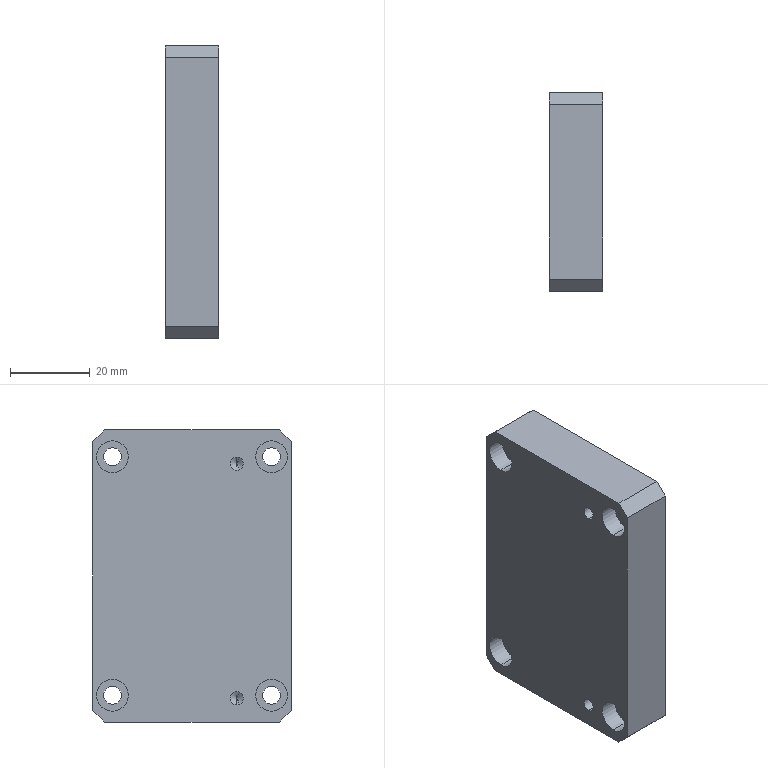Part | SolidWorks | features HoleWzd 3, Chamfer 1, Extrusion 1 | 1 solid | 46 faces | box 13.5 x 50 x 73.5 mm | volume 47539 mm3 | cylinder 24 | plane 14 | cone 8 | commonest cylinder face diameters 4.5 x8 8 x8 3.3 x4 4 x4
STEP:
#1=CARTESIAN_POINT('',(10.1,-11.25,26.6));
#2=VERTEX_POINT('',#1);
#3=CARTESIAN_POINT('',(10.1,-11.25,29.9));
#4=VERTEX_POINT('',#3);
#5=CARTESIAN_POINT('',(10.1,-11.25,28.25));
#6=DIRECTION('',(-1.,0.,0.));
#7=DIRECTION('',(0.,0.,1.));
#8=AXIS2_PLACEMENT_3D('',#5,#6,#7);
#9=CIRCLE('',#8,1.65);
#10=EDGE_CURVE('',#2,#4,#9,.T.);
#11=ORIENTED_EDGE('',*,*,#10,.F.);
#12=CARTESIAN_POINT('',(0.,-11.25,26.6));
#13=VERTEX_POINT('',#12);
#14=CARTESIAN_POINT('',(0.,-11.25,26.6));
#15=DIRECTION('',(-1.,0.,0.));
#16=VECTOR('',#15,1000.);
#17=LINE('',#14,#16);
#18=EDGE_CURVE('',#2,#13,#17,.T.);
#19=ORIENTED_EDGE('',*,*,#18,.T.);
#20=CARTESIAN_POINT('',(0.,-11.25,29.9));
#21=VERTEX_POINT('',#20);
#22=CARTESIAN_POINT('',(0.,-11.25,28.25));
#23=DIRECTION('',(-1.,0.,0.));
#24=DIRECTION('',(0.,0.,1.));
#25=AXIS2_PLACEMENT_3D('',#22,#23,#24);
#26=CIRCLE('',#25,1.65);
#27=EDGE_CURVE('',#13,#21,#26,.T.);
#28=ORIENTED_EDGE('',*,*,#27,.T.);
#29=CARTESIAN_POINT('',(0.,-11.25,29.9));
#30=DIRECTION('',(-1.,0.,0.));
#31=VECTOR('',#30,1000.);
#32=LINE('',#29,#31);
#33=EDGE_CURVE('',#4,#21,#32,.T.);
#34=ORIENTED_EDGE('',*,*,#33,.F.);
#35=EDGE_LOOP('',(#11,#19,#28,#34));
#36=FACE_OUTER_BOUND('',#35,.T.);
#37=CARTESIAN_POINT('',(0.,-11.25,28.25));
#38=DIRECTION('',(-1.,0.,0.));
#39=DIRECTION('',(0.,0.,1.));
#40=AXIS2_PLACEMENT_3D('',#37,#38,#39);
#41=CYLINDRICAL_SURFACE('',#40,1.65);
#42=ADVANCED_FACE('',(#36),#41,.F.);
#43=CARTESIAN_POINT('',(11.091,-11.25,28.25));
#44=VERTEX_POINT('',#43);
#45=CARTESIAN_POINT('',(10.1,-11.25,29.9));
#46=DIRECTION('',(-0.515,0.,0.8572));
#47=VECTOR('',#46,1000.);
#48=LINE('',#45,#47);
#49=EDGE_CURVE('',#44,#4,#48,.T.);
#50=ORIENTED_EDGE('',*,*,#49,.F.);
#51=CARTESIAN_POINT('',(10.1,-11.25,26.6));
#52=DIRECTION('',(-0.515,0.,-0.8572));
#53=VECTOR('',#52,1000.);
#54=LINE('',#51,#53);
#55=EDGE_CURVE('',#44,#2,#54,.T.);
#56=ORIENTED_EDGE('',*,*,#55,.T.);
#57=ORIENTED_EDGE('',*,*,#10,.T.);
#58=EDGE_LOOP('',(#50,#56,#57));
#59=FACE_OUTER_BOUND('',#58,.T.);
#60=CARTESIAN_POINT('',(10.1,-11.25,28.25));
#61=DIRECTION('',(-1.,0.,0.));
#62=DIRECTION('',(0.,0.,1.));
#63=AXIS2_PLACEMENT_3D('',#60,#61,#62);
#64=CONICAL_SURFACE('',#63,1.65,1.03);
#65=ADVANCED_FACE('',(#59),#64,.F.);
#66=CARTESIAN_POINT('',(10.1,-11.25,-32.4));
#67=VERTEX_POINT('',#66);
#68=CARTESIAN_POINT('',(10.1,-11.25,-29.1));
#69=VERTEX_POINT('',#68);
#70=CARTESIAN_POINT('',(10.1,-11.25,-30.75));
#71=DIRECTION('',(-1.,0.,0.));
#72=DIRECTION('',(0.,0.,1.));
#73=AXIS2_PLACEMENT_3D('',#70,#71,#72);
#74=CIRCLE('',#73,1.65);
#75=EDGE_CURVE('',#67,#69,#74,.T.);
#76=ORIENTED_EDGE('',*,*,#75,.F.);
#77=CARTESIAN_POINT('',(0.,-11.25,-32.4));
#78=VERTEX_POINT('',#77);
#79=CARTESIAN_POINT('',(0.,-11.25,-32.4));
#80=DIRECTION('',(-1.,0.,0.));
#81=VECTOR('',#80,1000.);
#82=LINE('',#79,#81);
#83=EDGE_CURVE('',#67,#78,#82,.T.);
#84=ORIENTED_EDGE('',*,*,#83,.T.);
#85=CARTESIAN_POINT('',(0.,-11.25,-29.1));
#86=VERTEX_POINT('',#85);
#87=CARTESIAN_POINT('',(0.,-11.25,-30.75));
#88=DIRECTION('',(-1.,0.,0.));
#89=DIRECTION('',(0.,0.,1.));
#90=AXIS2_PLACEMENT_3D('',#87,#88,#89);
#91=CIRCLE('',#90,1.65);
#92=EDGE_CURVE('',#78,#86,#91,.T.);
#93=ORIENTED_EDGE('',*,*,#92,.T.);
#94=CARTESIAN_POINT('',(0.,-11.25,-29.1));
#95=DIRECTION('',(-1.,0.,0.));
#96=VECTOR('',#95,1000.);
#97=LINE('',#94,#96);
#98=EDGE_CURVE('',#69,#86,#97,.T.);
#99=ORIENTED_EDGE('',*,*,#98,.F.);
#100=EDGE_LOOP('',(#76,#84,#93,#99));
#101=FACE_OUTER_BOUND('',#100,.T.);
#102=CARTESIAN_POINT('',(0.,-11.25,-30.75));
#103=DIRECTION('',(-1.,0.,0.));
#104=DIRECTION('',(0.,0.,1.));
#105=AXIS2_PLACEMENT_3D('',#102,#103,#104);
#106=CYLINDRICAL_SURFACE('',#105,1.65);
#107=ADVANCED_FACE('',(#101),#106,.F.);
#108=CARTESIAN_POINT('',(11.091,-11.25,-30.75));
#109=VERTEX_POINT('',#108);
#110=CARTESIAN_POINT('',(10.1,-11.25,-29.1));
#111=DIRECTION('',(-0.515,0.,0.8572));
#112=VECTOR('',#111,1000.);
#113=LINE('',#110,#112);
#114=EDGE_CURVE('',#109,#69,#113,.T.);
#115=ORIENTED_EDGE('',*,*,#114,.F.);
#116=CARTESIAN_POINT('',(10.1,-11.25,-32.4));
#117=DIRECTION('',(-0.515,0.,-0.8572));
#118=VECTOR('',#117,1000.);
#119=LINE('',#116,#118);
#120=EDGE_CURVE('',#109,#67,#119,.T.);
#121=ORIENTED_EDGE('',*,*,#120,.T.);
#122=ORIENTED_EDGE('',*,*,#75,.T.);
#123=EDGE_LOOP('',(#115,#121,#122));
#124=FACE_OUTER_BOUND('',#123,.T.);
#125=CARTESIAN_POINT('',(10.1,-11.25,-30.75));
#126=DIRECTION('',(-1.,0.,0.));
#127=DIRECTION('',(0.,0.,1.));
#128=AXIS2_PLACEMENT_3D('',#125,#126,#127);
#129=CONICAL_SURFACE('',#128,1.65,1.03);
#130=ADVANCED_FACE('',(#124),#129,.F.);
#131=CARTESIAN_POINT('',(7.5,0.,32.));
#132=VERTEX_POINT('',#131);
#133=CARTESIAN_POINT('',(7.5,0.,28.));
#134=VERTEX_POINT('',#133);
#135=CARTESIAN_POINT('',(7.5,0.,30.));
#136=DIRECTION('',(1.,0.,0.));
#137=DIRECTION('',(0.,0.,-1.));
#138=AXIS2_PLACEMENT_3D('',#135,#136,#137);
#139=CIRCLE('',#138,2.);
#140=EDGE_CURVE('',#132,#134,#139,.T.);
#141=ORIENTED_EDGE('',*,*,#140,.F.);
#142=CARTESIAN_POINT('',(13.5,0.,32.));
#143=VERTEX_POINT('',#142);
#144=CARTESIAN_POINT('',(13.5,0.,32.));
#145=DIRECTION('',(1.,0.,0.));
#146=VECTOR('',#145,1000.);
#147=LINE('',#144,#146);
#148=EDGE_CURVE('',#132,#143,#147,.T.);
#149=ORIENTED_EDGE('',*,*,#148,.T.);
#150=CARTESIAN_POINT('',(13.5,0.,28.));
#151=VERTEX_POINT('',#150);
#152=CARTESIAN_POINT('',(13.5,0.,30.));
#153=DIRECTION('',(1.,0.,0.));
#154=DIRECTION('',(0.,0.,-1.));
#155=AXIS2_PLACEMENT_3D('',#152,#153,#154);
#156=CIRCLE('',#155,2.);
#157=EDGE_CURVE('',#143,#151,#156,.T.);
#158=ORIENTED_EDGE('',*,*,#157,.T.);
#159=CARTESIAN_POINT('',(13.5,0.,28.));
#160=DIRECTION('',(1.,0.,0.));
#161=VECTOR('',#160,1000.);
#162=LINE('',#159,#161);
#163=EDGE_CURVE('',#134,#151,#162,.T.);
#164=ORIENTED_EDGE('',*,*,#163,.F.);
#165=EDGE_LOOP('',(#141,#149,#158,#164));
#166=FACE_OUTER_BOUND('',#165,.T.);
#167=CARTESIAN_POINT('',(13.5,0.,30.));
#168=DIRECTION('',(1.,0.,0.));
#169=DIRECTION('',(0.,0.,-1.));
#170=AXIS2_PLACEMENT_3D('',#167,#168,#169);
#171=CYLINDRICAL_SURFACE('',#170,2.);
#172=ADVANCED_FACE('',(#166),#171,.F.);
#173=CARTESIAN_POINT('',(6.298,0.,30.));
#174=VERTEX_POINT('',#173);
#175=CARTESIAN_POINT('',(7.5,0.,28.));
#176=DIRECTION('',(0.515,0.,-0.8572));
#177=VECTOR('',#176,1000.);
#178=LINE('',#175,#177);
#179=EDGE_CURVE('',#174,#134,#178,.T.);
#180=ORIENTED_EDGE('',*,*,#179,.F.);
#181=CARTESIAN_POINT('',(7.5,0.,32.));
#182=DIRECTION('',(0.515,0.,0.8572));
#183=VECTOR('',#182,1000.);
#184=LINE('',#181,#183);
#185=EDGE_CURVE('',#174,#132,#184,.T.);
#186=ORIENTED_EDGE('',*,*,#185,.T.);
#187=ORIENTED_EDGE('',*,*,#140,.T.);
#188=EDGE_LOOP('',(#180,#186,#187));
#189=FACE_OUTER_BOUND('',#188,.T.);
#190=CARTESIAN_POINT('',(7.5,0.,30.));
#191=DIRECTION('',(1.,0.,0.));
#192=DIRECTION('',(0.,0.,-1.));
#193=AXIS2_PLACEMENT_3D('',#190,#191,#192);
#194=CONICAL_SURFACE('',#193,2.,1.03);
#195=ADVANCED_FACE('',(#189),#194,.F.);
#196=CARTESIAN_POINT('',(7.5,0.,-28.));
#197=VERTEX_POINT('',#196);
#198=CARTESIAN_POINT('',(7.5,0.,-32.));
#199=VERTEX_POINT('',#198);
#200=CARTESIAN_POINT('',(7.5,0.,-30.));
#201=DIRECTION('',(1.,0.,0.));
#202=DIRECTION('',(0.,0.,-1.));
#203=AXIS2_PLACEMENT_3D('',#200,#201,#202);
#204=CIRCLE('',#203,2.);
#205=EDGE_CURVE('',#197,#199,#204,.T.);
#206=ORIENTED_EDGE('',*,*,#205,.F.);
#207=CARTESIAN_POINT('',(13.5,0.,-28.));
#208=VERTEX_POINT('',#207);
#209=CARTESIAN_POINT('',(13.5,0.,-28.));
#210=DIRECTION('',(1.,0.,0.));
#211=VECTOR('',#210,1000.);
#212=LINE('',#209,#211);
#213=EDGE_CURVE('',#197,#208,#212,.T.);
#214=ORIENTED_EDGE('',*,*,#213,.T.);
#215=CARTESIAN_POINT('',(13.5,0.,-32.));
#216=VERTEX_POINT('',#215);
#217=CARTESIAN_POINT('',(13.5,0.,-30.));
#218=DIRECTION('',(1.,0.,0.));
#219=DIRECTION('',(0.,0.,-1.));
#220=AXIS2_PLACEMENT_3D('',#217,#218,#219);
#221=CIRCLE('',#220,2.);
#222=EDGE_CURVE('',#208,#216,#221,.T.);
#223=ORIENTED_EDGE('',*,*,#222,.T.);
#224=CARTESIAN_POINT('',(13.5,0.,-32.));
#225=DIRECTION('',(1.,0.,0.));
#226=VECTOR('',#225,1000.);
#227=LINE('',#224,#226);
#228=EDGE_CURVE('',#199,#216,#227,.T.);
#229=ORIENTED_EDGE('',*,*,#228,.F.);
#230=EDGE_LOOP('',(#206,#214,#223,#229));
#231=FACE_OUTER_BOUND('',#230,.T.);
#232=CARTESIAN_POINT('',(13.5,0.,-30.));
#233=DIRECTION('',(1.,0.,0.));
#234=DIRECTION('',(0.,0.,-1.));
#235=AXIS2_PLACEMENT_3D('',#232,#233,#234);
#236=CYLINDRICAL_SURFACE('',#235,2.);
#237=ADVANCED_FACE('',(#231),#236,.F.);
#238=CARTESIAN_POINT('',(6.298,0.,-30.));
#239=VERTEX_POINT('',#238);
#240=CARTESIAN_POINT('',(7.5,0.,-32.));
#241=DIRECTION('',(0.515,0.,-0.8572));
#242=VECTOR('',#241,1000.);
#243=LINE('',#240,#242);
#244=EDGE_CURVE('',#239,#199,#243,.T.);
#245=ORIENTED_EDGE('',*,*,#244,.F.);
#246=CARTESIAN_POINT('',(7.5,0.,-28.));
#247=DIRECTION('',(0.515,0.,0.8572));
#248=VECTOR('',#247,1000.);
#249=LINE('',#246,#248);
#250=EDGE_CURVE('',#239,#197,#249,.T.);
#251=ORIENTED_EDGE('',*,*,#250,.T.);
#252=ORIENTED_EDGE('',*,*,#205,.T.);
#253=EDGE_LOOP('',(#245,#251,#252));
#254=FACE_OUTER_BOUND('',#253,.T.);
#255=CARTESIAN_POINT('',(7.5,0.,-30.));
#256=DIRECTION('',(1.,0.,0.));
#257=DIRECTION('',(0.,0.,-1.));
#258=AXIS2_PLACEMENT_3D('',#255,#256,#257);
#259=CONICAL_SURFACE('',#258,2.,1.03);
#260=ADVANCED_FACE('',(#254),#259,.F.);
#261=CARTESIAN_POINT('',(4.6,20.,26.));
#262=VERTEX_POINT('',#261);
#263=CARTESIAN_POINT('',(4.6,20.,34.));
#264=VERTEX_POINT('',#263);
#265=CARTESIAN_POINT('',(4.6,20.,30.));
#266=DIRECTION('',(-1.,0.,0.));
#267=DIRECTION('',(0.,0.,1.));
#268=AXIS2_PLACEMENT_3D('',#265,#266,#267);
#269=CIRCLE('',#268,4.);
#270=EDGE_CURVE('',#262,#264,#269,.T.);
#271=ORIENTED_EDGE('',*,*,#270,.F.);
#272=CARTESIAN_POINT('',(0.,20.,26.));
#273=VERTEX_POINT('',#272);
#274=CARTESIAN_POINT('',(0.,20.,26.));
#275=DIRECTION('',(-1.,0.,0.));
#276=VECTOR('',#275,1000.);
#277=LINE('',#274,#276);
#278=EDGE_CURVE('',#262,#273,#277,.T.);
#279=ORIENTED_EDGE('',*,*,#278,.T.);
#280=CARTESIAN_POINT('',(0.,20.,34.));
#281=VERTEX_POINT('',#280);
#282=CARTESIAN_POINT('',(0.,20.,30.));
#283=DIRECTION('',(-1.,0.,0.));
#284=DIRECTION('',(0.,0.,1.));
#285=AXIS2_PLACEMENT_3D('',#282,#283,#284);
#286=CIRCLE('',#285,4.);
#287=EDGE_CURVE('',#273,#281,#286,.T.);
#288=ORIENTED_EDGE('',*,*,#287,.T.);
#289=CARTESIAN_POINT('',(0.,20.,34.));
#290=DIRECTION('',(-1.,0.,0.));
#291=VECTOR('',#290,1000.);
#292=LINE('',#289,#291);
#293=EDGE_CURVE('',#264,#281,#292,.T.);
#294=ORIENTED_EDGE('',*,*,#293,.F.);
#295=EDGE_LOOP('',(#271,#279,#288,#294));
#296=FACE_OUTER_BOUND('',#295,.T.);
#297=CARTESIAN_POINT('',(0.,20.,30.));
#298=DIRECTION('',(-1.,0.,0.));
#299=DIRECTION('',(0.,0.,1.));
#300=AXIS2_PLACEMENT_3D('',#297,#298,#299);
#301=CYLINDRICAL_SURFACE('',#300,4.);
#302=ADVANCED_FACE('',(#296),#301,.F.);
#303=CARTESIAN_POINT('',(13.5,20.,27.75));
#304=VERTEX_POINT('',#303);
#305=CARTESIAN_POINT('',(13.5,20.,32.25));
#306=VERTEX_POINT('',#305);
#307=CARTESIAN_POINT('',(13.5,20.,30.));
#308=DIRECTION('',(-1.,0.,0.));
#309=DIRECTION('',(0.,0.,1.));
#310=AXIS2_PLACEMENT_3D('',#307,#308,#309);
#311=CIRCLE('',#310,2.25);
#312=EDGE_CURVE('',#304,#306,#311,.T.);
#313=ORIENTED_EDGE('',*,*,#312,.F.);
#314=CARTESIAN_POINT('',(4.6,20.,27.75));
#315=VERTEX_POINT('',#314);
#316=CARTESIAN_POINT('',(0.,20.,27.75));
#317=DIRECTION('',(-1.,0.,0.));
#318=VECTOR('',#317,1000.);
#319=LINE('',#316,#318);
#320=EDGE_CURVE('',#304,#315,#319,.T.);
#321=ORIENTED_EDGE('',*,*,#320,.T.);
#322=CARTESIAN_POINT('',(4.6,20.,32.25));
#323=VERTEX_POINT('',#322);
#324=CARTESIAN_POINT('',(4.6,20.,30.));
#325=DIRECTION('',(-1.,0.,0.));
#326=DIRECTION('',(0.,0.,1.));
#327=AXIS2_PLACEMENT_3D('',#324,#325,#326);
#328=CIRCLE('',#327,2.25);
#329=EDGE_CURVE('',#315,#323,#328,.T.);
#330=ORIENTED_EDGE('',*,*,#329,.T.);
#331=CARTESIAN_POINT('',(0.,20.,32.25));
#332=DIRECTION('',(-1.,0.,0.));
#333=VECTOR('',#332,1000.);
#334=LINE('',#331,#333);
#335=EDGE_CURVE('',#306,#323,#334,.T.);
#336=ORIENTED_EDGE('',*,*,#335,.F.);
#337=EDGE_LOOP('',(#313,#321,#330,#336));
#338=FACE_OUTER_BOUND('',#337,.T.);
#339=CARTESIAN_POINT('',(0.,20.,30.));
#340=DIRECTION('',(-1.,0.,0.));
#341=DIRECTION('',(0.,0.,1.));
#342=AXIS2_PLACEMENT_3D('',#339,#340,#341);
#343=CYLINDRICAL_SURFACE('',#342,2.25);
#344=ADVANCED_FACE('',(#338),#343,.F.);
#345=CARTESIAN_POINT('',(4.6,20.,-34.));
#346=VERTEX_POINT('',#345);
#347=CARTESIAN_POINT('',(4.6,20.,-26.));
#348=VERTEX_POINT('',#347);
#349=CARTESIAN_POINT('',(4.6,20.,-30.));
#350=DIRECTION('',(-1.,0.,0.));
#351=DIRECTION('',(0.,0.,1.));
#352=AXIS2_PLACEMENT_3D('',#349,#350,#351);
#353=CIRCLE('',#352,4.);
#354=EDGE_CURVE('',#346,#348,#353,.T.);
#355=ORIENTED_EDGE('',*,*,#354,.F.);
#356=CARTESIAN_POINT('',(0.,20.,-34.));
#357=VERTEX_POINT('',#356);
#358=CARTESIAN_POINT('',(0.,20.,-34.));
#359=DIRECTION('',(-1.,0.,0.));
#360=VECTOR('',#359,1000.);
#361=LINE('',#358,#360);
#362=EDGE_CURVE('',#346,#357,#361,.T.);
#363=ORIENTED_EDGE('',*,*,#362,.T.);
#364=CARTESIAN_POINT('',(0.,20.,-26.));
#365=VERTEX_POINT('',#364);
#366=CARTESIAN_POINT('',(0.,20.,-30.));
#367=DIRECTION('',(-1.,0.,0.));
#368=DIRECTION('',(0.,0.,1.));
#369=AXIS2_PLACEMENT_3D('',#366,#367,#368);
#370=CIRCLE('',#369,4.);
#371=EDGE_CURVE('',#357,#365,#370,.T.);
#372=ORIENTED_EDGE('',*,*,#371,.T.);
#373=CARTESIAN_POINT('',(0.,20.,-26.));
#374=DIRECTION('',(-1.,0.,0.));
#375=VECTOR('',#374,1000.);
#376=LINE('',#373,#375);
#377=EDGE_CURVE('',#348,#365,#376,.T.);
#378=ORIENTED_EDGE('',*,*,#377,.F.);
#379=EDGE_LOOP('',(#355,#363,#372,#378));
#380=FACE_OUTER_BOUND('',#379,.T.);
#381=CARTESIAN_POINT('',(0.,20.,-30.));
#382=DIRECTION('',(-1.,0.,0.));
#383=DIRECTION('',(0.,0.,1.));
#384=AXIS2_PLACEMENT_3D('',#381,#382,#383);
#385=CYLINDRICAL_SURFACE('',#384,4.);
#386=ADVANCED_FACE('',(#380),#385,.F.);
#387=CARTESIAN_POINT('',(13.5,20.,-32.25));
#388=VERTEX_POINT('',#387);
#389=CARTESIAN_POINT('',(13.5,20.,-27.75));
#390=VERTEX_POINT('',#389);
#391=CARTESIAN_POINT('',(13.5,20.,-30.));
#392=DIRECTION('',(-1.,0.,0.));
#393=DIRECTION('',(0.,0.,1.));
#394=AXIS2_PLACEMENT_3D('',#391,#392,#393);
#395=CIRCLE('',#394,2.25);
#396=EDGE_CURVE('',#388,#390,#395,.T.);
#397=ORIENTED_EDGE('',*,*,#396,.F.);
#398=CARTESIAN_POINT('',(4.6,20.,-32.25));
#399=VERTEX_POINT('',#398);
#400=CARTESIAN_POINT('',(0.,20.,-32.25));
#401=DIRECTION('',(-1.,0.,0.));
#402=VECTOR('',#401,1000.);
#403=LINE('',#400,#402);
#404=EDGE_CURVE('',#388,#399,#403,.T.);
#405=ORIENTED_EDGE('',*,*,#404,.T.);
#406=CARTESIAN_POINT('',(4.6,20.,-27.75));
#407=VERTEX_POINT('',#406);
#408=CARTESIAN_POINT('',(4.6,20.,-30.));
#409=DIRECTION('',(-1.,0.,0.));
#410=DIRECTION('',(0.,0.,1.));
#411=AXIS2_PLACEMENT_3D('',#408,#409,#410);
#412=CIRCLE('',#411,2.25);
#413=EDGE_CURVE('',#399,#407,#412,.T.);
#414=ORIENTED_EDGE('',*,*,#413,.T.);
#415=CARTESIAN_POINT('',(0.,20.,-27.75));
#416=DIRECTION('',(-1.,0.,0.));
#417=VECTOR('',#416,1000.);
#418=LINE('',#415,#417);
#419=EDGE_CURVE('',#390,#407,#418,.T.);
#420=ORIENTED_EDGE('',*,*,#419,.F.);
#421=EDGE_LOOP('',(#397,#405,#414,#420));
#422=FACE_OUTER_BOUND('',#421,.T.);
#423=CARTESIAN_POINT('',(0.,20.,-30.));
#424=DIRECTION('',(-1.,0.,0.));
#425=DIRECTION('',(0.,0.,1.));
#426=AXIS2_PLACEMENT_3D('',#423,#424,#425);
#427=CYLINDRICAL_SURFACE('',#426,2.25);
#428=ADVANCED_FACE('',(#422),#427,.F.);
#429=CARTESIAN_POINT('',(4.6,-20.,-34.));
#430=VERTEX_POINT('',#429);
#431=CARTESIAN_POINT('',(4.6,-20.,-26.));
#432=VERTEX_POINT('',#431);
#433=CARTESIAN_POINT('',(4.6,-20.,-30.));
#434=DIRECTION('',(-1.,0.,0.));
#435=DIRECTION('',(0.,0.,1.));
#436=AXIS2_PLACEMENT_3D('',#433,#434,#435);
#437=CIRCLE('',#436,4.);
#438=EDGE_CURVE('',#430,#432,#437,.T.);
#439=ORIENTED_EDGE('',*,*,#438,.F.);
#440=CARTESIAN_POINT('',(0.,-20.,-34.));
#441=VERTEX_POINT('',#440);
#442=CARTESIAN_POINT('',(0.,-20.,-34.));
#443=DIRECTION('',(-1.,0.,0.));
#444=VECTOR('',#443,1000.);
#445=LINE('',#442,#444);
#446=EDGE_CURVE('',#430,#441,#445,.T.);
#447=ORIENTED_EDGE('',*,*,#446,.T.);
#448=CARTESIAN_POINT('',(0.,-20.,-26.));
#449=VERTEX_POINT('',#448);
#450=CARTESIAN_POINT('',(0.,-20.,-30.));
#451=DIRECTION('',(-1.,0.,0.));
#452=DIRECTION('',(0.,0.,1.));
#453=AXIS2_PLACEMENT_3D('',#450,#451,#452);
#454=CIRCLE('',#453,4.);
#455=EDGE_CURVE('',#441,#449,#454,.T.);
#456=ORIENTED_EDGE('',*,*,#455,.T.);
#457=CARTESIAN_POINT('',(0.,-20.,-26.));
#458=DIRECTION('',(-1.,0.,0.));
#459=VECTOR('',#458,1000.);
#460=LINE('',#457,#459);
#461=EDGE_CURVE('',#432,#449,#460,.T.);
#462=ORIENTED_EDGE('',*,*,#461,.F.);
#463=EDGE_LOOP('',(#439,#447,#456,#462));
#464=FACE_OUTER_BOUND('',#463,.T.);
#465=CARTESIAN_POINT('',(0.,-20.,-30.));
#466=DIRECTION('',(-1.,0.,0.));
#467=DIRECTION('',(0.,0.,1.));
#468=AXIS2_PLACEMENT_3D('',#465,#466,#467);
#469=CYLINDRICAL_SURFACE('',#468,4.);
#470=ADVANCED_FACE('',(#464),#469,.F.);
#471=CARTESIAN_POINT('',(13.5,-20.,-32.25));
#472=VERTEX_POINT('',#471);
#473=CARTESIAN_POINT('',(13.5,-20.,-27.75));
#474=VERTEX_POINT('',#473);
#475=CARTESIAN_POINT('',(13.5,-20.,-30.));
#476=DIRECTION('',(-1.,0.,0.));
#477=DIRECTION('',(0.,0.,1.));
#478=AXIS2_PLACEMENT_3D('',#475,#476,#477);
#479=CIRCLE('',#478,2.25);
#480=EDGE_CURVE('',#472,#474,#479,.T.);
#481=ORIENTED_EDGE('',*,*,#480,.F.);
#482=CARTESIAN_POINT('',(4.6,-20.,-32.25));
#483=VERTEX_POINT('',#482);
#484=CARTESIAN_POINT('',(0.,-20.,-32.25));
#485=DIRECTION('',(-1.,0.,0.));
#486=VECTOR('',#485,1000.);
#487=LINE('',#484,#486);
#488=EDGE_CURVE('',#472,#483,#487,.T.);
#489=ORIENTED_EDGE('',*,*,#488,.T.);
#490=CARTESIAN_POINT('',(4.6,-20.,-27.75));
#491=VERTEX_POINT('',#490);
#492=CARTESIAN_POINT('',(4.6,-20.,-30.));
#493=DIRECTION('',(-1.,0.,0.));
#494=DIRECTION('',(0.,0.,1.));
#495=AXIS2_PLACEMENT_3D('',#492,#493,#494);
#496=CIRCLE('',#495,2.25);
#497=EDGE_CURVE('',#483,#491,#496,.T.);
#498=ORIENTED_EDGE('',*,*,#497,.T.);
#499=CARTESIAN_POINT('',(0.,-20.,-27.75));
#500=DIRECTION('',(-1.,0.,0.));
#501=VECTOR('',#500,1000.);
#502=LINE('',#499,#501);
#503=EDGE_CURVE('',#474,#491,#502,.T.);
#504=ORIENTED_EDGE('',*,*,#503,.F.);
#505=EDGE_LOOP('',(#481,#489,#498,#504));
#506=FACE_OUTER_BOUND('',#505,.T.);
#507=CARTESIAN_POINT('',(0.,-20.,-30.));
#508=DIRECTION('',(-1.,0.,0.));
#509=DIRECTION('',(0.,0.,1.));
#510=AXIS2_PLACEMENT_3D('',#507,#508,#509);
#511=CYLINDRICAL_SURFACE('',#510,2.25);
#512=ADVANCED_FACE('',(#506),#511,.F.);
#513=CARTESIAN_POINT('',(4.6,-20.,26.));
#514=VERTEX_POINT('',#513);
#515=CARTESIAN_POINT('',(4.6,-20.,34.));
#516=VERTEX_POINT('',#515);
#517=CARTESIAN_POINT('',(4.6,-20.,30.));
#518=DIRECTION('',(-1.,0.,0.));
#519=DIRECTION('',(0.,0.,1.));
#520=AXIS2_PLACEMENT_3D('',#517,#518,#519);
#521=CIRCLE('',#520,4.);
#522=EDGE_CURVE('',#514,#516,#521,.T.);
#523=ORIENTED_EDGE('',*,*,#522,.F.);
#524=CARTESIAN_POINT('',(0.,-20.,26.));
#525=VERTEX_POINT('',#524);
#526=CARTESIAN_POINT('',(0.,-20.,26.));
#527=DIRECTION('',(-1.,0.,0.));
#528=VECTOR('',#527,1000.);
#529=LINE('',#526,#528);
#530=EDGE_CURVE('',#514,#525,#529,.T.);
#531=ORIENTED_EDGE('',*,*,#530,.T.);
#532=CARTESIAN_POINT('',(0.,-20.,34.));
#533=VERTEX_POINT('',#532);
#534=CARTESIAN_POINT('',(0.,-20.,30.));
#535=DIRECTION('',(-1.,0.,0.));
#536=DIRECTION('',(0.,0.,1.));
#537=AXIS2_PLACEMENT_3D('',#534,#535,#536);
#538=CIRCLE('',#537,4.);
#539=EDGE_CURVE('',#525,#533,#538,.T.);
#540=ORIENTED_EDGE('',*,*,#539,.T.);
#541=CARTESIAN_POINT('',(0.,-20.,34.));
#542=DIRECTION('',(-1.,0.,0.));
#543=VECTOR('',#542,1000.);
#544=LINE('',#541,#543);
#545=EDGE_CURVE('',#516,#533,#544,.T.);
#546=ORIENTED_EDGE('',*,*,#545,.F.);
#547=EDGE_LOOP('',(#523,#531,#540,#546));
#548=FACE_OUTER_BOUND('',#547,.T.);
#549=CARTESIAN_POINT('',(0.,-20.,30.));
#550=DIRECTION('',(-1.,0.,0.));
#551=DIRECTION('',(0.,0.,1.));
#552=AXIS2_PLACEMENT_3D('',#549,#550,#551);
#553=CYLINDRICAL_SURFACE('',#552,4.);
#554=ADVANCED_FACE('',(#548),#553,.F.);
#555=CARTESIAN_POINT('',(13.5,-20.,27.75));
#556=VERTEX_POINT('',#555);
#557=CARTESIAN_POINT('',(13.5,-20.,32.25));
#558=VERTEX_POINT('',#557);
#559=CARTESIAN_POINT('',(13.5,-20.,30.));
#560=DIRECTION('',(-1.,0.,0.));
#561=DIRECTION('',(0.,0.,1.));
#562=AXIS2_PLACEMENT_3D('',#559,#560,#561);
#563=CIRCLE('',#562,2.25);
#564=EDGE_CURVE('',#556,#558,#563,.T.);
#565=ORIENTED_EDGE('',*,*,#564,.F.);
#566=CARTESIAN_POINT('',(4.6,-20.,27.75));
#567=VERTEX_POINT('',#566);
#568=CARTESIAN_POINT('',(0.,-20.,27.75));
#569=DIRECTION('',(-1.,0.,0.));
#570=VECTOR('',#569,1000.);
#571=LINE('',#568,#570);
#572=EDGE_CURVE('',#556,#567,#571,.T.);
#573=ORIENTED_EDGE('',*,*,#572,.T.);
#574=CARTESIAN_POINT('',(4.6,-20.,32.25));
#575=VERTEX_POINT('',#574);
#576=CARTESIAN_POINT('',(4.6,-20.,30.));
#577=DIRECTION('',(-1.,0.,0.));
#578=DIRECTION('',(0.,0.,1.));
#579=AXIS2_PLACEMENT_3D('',#576,#577,#578);
#580=CIRCLE('',#579,2.25);
#581=EDGE_CURVE('',#567,#575,#580,.T.);
#582=ORIENTED_EDGE('',*,*,#581,.T.);
#583=CARTESIAN_POINT('',(0.,-20.,32.25));
#584=DIRECTION('',(-1.,0.,0.));
#585=VECTOR('',#584,1000.);
#586=LINE('',#583,#585);
#587=EDGE_CURVE('',#558,#575,#586,.T.);
#588=ORIENTED_EDGE('',*,*,#587,.F.);
#589=EDGE_LOOP('',(#565,#573,#582,#588));
#590=FACE_OUTER_BOUND('',#589,.T.);
#591=CARTESIAN_POINT('',(0.,-20.,30.));
#592=DIRECTION('',(-1.,0.,0.));
#593=DIRECTION('',(0.,0.,1.));
#594=AXIS2_PLACEMENT_3D('',#591,#592,#593);
#595=CYLINDRICAL_SURFACE('',#594,2.25);
#596=ADVANCED_FACE('',(#590),#595,.F.);
#597=CARTESIAN_POINT('',(13.5,-22.,-36.75));
#598=VERTEX_POINT('',#597);
#599=CARTESIAN_POINT('',(13.5,22.,-36.75));
#600=VERTEX_POINT('',#599);
#601=CARTESIAN_POINT('',(13.5,-25.,-36.75));
#602=DIRECTION('',(0.,1.,0.));
#603=VECTOR('',#602,1000.);
#604=LINE('',#601,#603);
#605=EDGE_CURVE('',#598,#600,#604,.T.);
#606=ORIENTED_EDGE('',*,*,#605,.F.);
#607=CARTESIAN_POINT('',(0.,-22.,-36.75));
#608=VERTEX_POINT('',#607);
#609=CARTESIAN_POINT('',(13.5,-22.,-36.75));
#610=DIRECTION('',(-1.,0.,0.));
#611=VECTOR('',#610,1000.);
#612=LINE('',#609,#611);
#613=EDGE_CURVE('',#598,#608,#612,.T.);
#614=ORIENTED_EDGE('',*,*,#613,.T.);
#615=CARTESIAN_POINT('',(0.,22.,-36.75));
#616=VERTEX_POINT('',#615);
#617=CARTESIAN_POINT('',(0.,-25.,-36.75));
#618=DIRECTION('',(0.,1.,0.));
#619=VECTOR('',#618,1000.);
#620=LINE('',#617,#619);
#621=EDGE_CURVE('',#608,#616,#620,.T.);
#622=ORIENTED_EDGE('',*,*,#621,.T.);
#623=CARTESIAN_POINT('',(13.5,22.,-36.75));
#624=DIRECTION('',(1.,0.,0.));
#625=VECTOR('',#624,1000.);
#626=LINE('',#623,#625);
#627=EDGE_CURVE('',#616,#600,#626,.T.);
#628=ORIENTED_EDGE('',*,*,#627,.T.);
#629=EDGE_LOOP('',(#606,#614,#622,#628));
#630=FACE_OUTER_BOUND('',#629,.T.);
#631=CARTESIAN_POINT('',(13.5,-25.,-36.75));
#632=DIRECTION('',(0.,0.,1.));
#633=DIRECTION('',(1.,0.,0.));
#634=AXIS2_PLACEMENT_3D('',#631,#632,#633);
#635=PLANE('',#634);
#636=ADVANCED_FACE('',(#630),#635,.F.);
#637=CARTESIAN_POINT('',(13.5,25.,-33.75));
#638=VERTEX_POINT('',#637);
#639=CARTESIAN_POINT('',(13.5,25.,33.75));
#640=VERTEX_POINT('',#639);
#641=CARTESIAN_POINT('',(13.5,25.,36.75));
#642=DIRECTION('',(0.,0.,1.));
#643=VECTOR('',#642,1000.);
#644=LINE('',#641,#643);
#645=EDGE_CURVE('',#638,#640,#644,.T.);
#646=ORIENTED_EDGE('',*,*,#645,.F.);
#647=CARTESIAN_POINT('',(0.,25.,-33.75));
#648=VERTEX_POINT('',#647);
#649=CARTESIAN_POINT('',(13.5,25.,-33.75));
#650=DIRECTION('',(-1.,0.,0.));
#651=VECTOR('',#650,1000.);
#652=LINE('',#649,#651);
#653=EDGE_CURVE('',#638,#648,#652,.T.);
#654=ORIENTED_EDGE('',*,*,#653,.T.);
#655=CARTESIAN_POINT('',(0.,25.,33.75));
#656=VERTEX_POINT('',#655);
#657=CARTESIAN_POINT('',(0.,25.,36.75));
#658=DIRECTION('',(0.,0.,1.));
#659=VECTOR('',#658,1000.);
#660=LINE('',#657,#659);
#661=EDGE_CURVE('',#648,#656,#660,.T.);
#662=ORIENTED_EDGE('',*,*,#661,.T.);
#663=CARTESIAN_POINT('',(13.5,25.,33.75));
#664=DIRECTION('',(1.,0.,0.));
#665=VECTOR('',#664,1000.);
#666=LINE('',#663,#665);
#667=EDGE_CURVE('',#656,#640,#666,.T.);
#668=ORIENTED_EDGE('',*,*,#667,.T.);
#669=EDGE_LOOP('',(#646,#654,#662,#668));
#670=FACE_OUTER_BOUND('',#669,.T.);
#671=CARTESIAN_POINT('',(13.5,25.,36.75));
#672=DIRECTION('',(0.,-1.,0.));
#673=DIRECTION('',(0.,0.,-1.));
#674=AXIS2_PLACEMENT_3D('',#671,#672,#673);
#675=PLANE('',#674);
#676=ADVANCED_FACE('',(#670),#675,.F.);
#677=CARTESIAN_POINT('',(0.,22.,36.75));
#678=VERTEX_POINT('',#677);
#679=CARTESIAN_POINT('',(0.,-22.,36.75));
#680=VERTEX_POINT('',#679);
#681=CARTESIAN_POINT('',(0.,-25.,36.75));
#682=DIRECTION('',(0.,-1.,0.));
#683=VECTOR('',#682,1000.);
#684=LINE('',#681,#683);
#685=EDGE_CURVE('',#678,#680,#684,.T.);
#686=ORIENTED_EDGE('',*,*,#685,.T.);
#687=CARTESIAN_POINT('',(13.5,-22.,36.75));
#688=VERTEX_POINT('',#687);
#689=CARTESIAN_POINT('',(13.5,-22.,36.75));
#690=DIRECTION('',(1.,0.,0.));
#691=VECTOR('',#690,1000.);
#692=LINE('',#689,#691);
#693=EDGE_CURVE('',#680,#688,#692,.T.);
#694=ORIENTED_EDGE('',*,*,#693,.T.);
#695=CARTESIAN_POINT('',(13.5,22.,36.75));
#696=VERTEX_POINT('',#695);
#697=CARTESIAN_POINT('',(13.5,-25.,36.75));
#698=DIRECTION('',(0.,-1.,0.));
#699=VECTOR('',#698,1000.);
#700=LINE('',#697,#699);
#701=EDGE_CURVE('',#696,#688,#700,.T.);
#702=ORIENTED_EDGE('',*,*,#701,.F.);
#703=CARTESIAN_POINT('',(13.5,22.,36.75));
#704=DIRECTION('',(-1.,0.,0.));
#705=VECTOR('',#704,1000.);
#706=LINE('',#703,#705);
#707=EDGE_CURVE('',#696,#678,#706,.T.);
#708=ORIENTED_EDGE('',*,*,#707,.T.);
#709=EDGE_LOOP('',(#686,#694,#702,#708));
#710=FACE_OUTER_BOUND('',#709,.T.);
#711=CARTESIAN_POINT('',(13.5,-25.,36.75));
#712=DIRECTION('',(0.,0.,-1.));
#713=DIRECTION('',(-1.,0.,0.));
#714=AXIS2_PLACEMENT_3D('',#711,#712,#713);
#715=PLANE('',#714);
#716=ADVANCED_FACE('',(#710),#715,.F.);
#717=CARTESIAN_POINT('',(0.,-25.,33.75));
#718=VERTEX_POINT('',#717);
#719=CARTESIAN_POINT('',(0.,-25.,-33.75));
#720=VERTEX_POINT('',#719);
#721=CARTESIAN_POINT('',(0.,-25.,36.75));
#722=DIRECTION('',(0.,0.,-1.));
#723=VECTOR('',#722,1000.);
#724=LINE('',#721,#723);
#725=EDGE_CURVE('',#718,#720,#724,.T.);
#726=ORIENTED_EDGE('',*,*,#725,.T.);
#727=CARTESIAN_POINT('',(13.5,-25.,-33.75));
#728=VERTEX_POINT('',#727);
#729=CARTESIAN_POINT('',(13.5,-25.,-33.75));
#730=DIRECTION('',(1.,0.,0.));
#731=VECTOR('',#730,1000.);
#732=LINE('',#729,#731);
#733=EDGE_CURVE('',#720,#728,#732,.T.);
#734=ORIENTED_EDGE('',*,*,#733,.T.);
#735=CARTESIAN_POINT('',(13.5,-25.,33.75));
#736=VERTEX_POINT('',#735);
#737=CARTESIAN_POINT('',(13.5,-25.,36.75));
#738=DIRECTION('',(0.,0.,-1.));
#739=VECTOR('',#738,1000.);
#740=LINE('',#737,#739);
#741=EDGE_CURVE('',#736,#728,#740,.T.);
#742=ORIENTED_EDGE('',*,*,#741,.F.);
#743=CARTESIAN_POINT('',(13.5,-25.,33.75));
#744=DIRECTION('',(-1.,0.,0.));
#745=VECTOR('',#744,1000.);
#746=LINE('',#743,#745);
#747=EDGE_CURVE('',#736,#718,#746,.T.);
#748=ORIENTED_EDGE('',*,*,#747,.T.);
#749=EDGE_LOOP('',(#726,#734,#742,#748));
#750=FACE_OUTER_BOUND('',#749,.T.);
#751=CARTESIAN_POINT('',(13.5,-25.,36.75));
#752=DIRECTION('',(0.,1.,0.));
#753=DIRECTION('',(0.,0.,1.));
#754=AXIS2_PLACEMENT_3D('',#751,#752,#753);
#755=PLANE('',#754);
#756=ADVANCED_FACE('',(#750),#755,.F.);
#757=CARTESIAN_POINT('',(13.5,0.,30.));
#758=DIRECTION('',(1.,0.,0.));
#759=DIRECTION('',(0.,0.,-1.));
#760=AXIS2_PLACEMENT_3D('',#757,#758,#759);
#761=CIRCLE('',#760,2.);
#762=EDGE_CURVE('',#151,#143,#761,.T.);
#763=ORIENTED_EDGE('',*,*,#762,.F.);
#764=ORIENTED_EDGE('',*,*,#157,.F.);
#765=EDGE_LOOP('',(#763,#764));
#766=FACE_BOUND('',#765,.T.);
#767=CARTESIAN_POINT('',(13.5,0.,-30.));
#768=DIRECTION('',(1.,0.,0.));
#769=DIRECTION('',(0.,0.,-1.));
#770=AXIS2_PLACEMENT_3D('',#767,#768,#769);
#771=CIRCLE('',#770,2.);
#772=EDGE_CURVE('',#216,#208,#771,.T.);
#773=ORIENTED_EDGE('',*,*,#772,.F.);
#774=ORIENTED_EDGE('',*,*,#222,.F.);
#775=EDGE_LOOP('',(#773,#774));
#776=FACE_BOUND('',#775,.T.);
#777=CARTESIAN_POINT('',(13.5,20.,30.));
#778=DIRECTION('',(-1.,0.,0.));
#779=DIRECTION('',(0.,0.,1.));
#780=AXIS2_PLACEMENT_3D('',#777,#778,#779);
#781=CIRCLE('',#780,2.25);
#782=EDGE_CURVE('',#306,#304,#781,.T.);
#783=ORIENTED_EDGE('',*,*,#782,.T.);
#784=ORIENTED_EDGE('',*,*,#312,.T.);
#785=EDGE_LOOP('',(#783,#784));
#786=FACE_BOUND('',#785,.T.);
#787=CARTESIAN_POINT('',(13.5,20.,-30.));
#788=DIRECTION('',(-1.,0.,0.));
#789=DIRECTION('',(0.,0.,1.));
#790=AXIS2_PLACEMENT_3D('',#787,#788,#789);
#791=CIRCLE('',#790,2.25);
#792=EDGE_CURVE('',#390,#388,#791,.T.);
#793=ORIENTED_EDGE('',*,*,#792,.T.);
#794=ORIENTED_EDGE('',*,*,#396,.T.);
#795=EDGE_LOOP('',(#793,#794));
#796=FACE_BOUND('',#795,.T.);
#797=CARTESIAN_POINT('',(13.5,-20.,-30.));
#798=DIRECTION('',(-1.,0.,0.));
#799=DIRECTION('',(0.,0.,1.));
#800=AXIS2_PLACEMENT_3D('',#797,#798,#799);
#801=CIRCLE('',#800,2.25);
#802=EDGE_CURVE('',#474,#472,#801,.T.);
#803=ORIENTED_EDGE('',*,*,#802,.T.);
#804=ORIENTED_EDGE('',*,*,#480,.T.);
#805=EDGE_LOOP('',(#803,#804));
#806=FACE_BOUND('',#805,.T.);
#807=CARTESIAN_POINT('',(13.5,-20.,30.));
#808=DIRECTION('',(-1.,0.,0.));
#809=DIRECTION('',(0.,0.,1.));
#810=AXIS2_PLACEMENT_3D('',#807,#808,#809);
#811=CIRCLE('',#810,2.25);
#812=EDGE_CURVE('',#558,#556,#811,.T.);
#813=ORIENTED_EDGE('',*,*,#812,.T.);
#814=ORIENTED_EDGE('',*,*,#564,.T.);
#815=EDGE_LOOP('',(#813,#814));
#816=FACE_BOUND('',#815,.T.);
#817=ORIENTED_EDGE('',*,*,#741,.T.);
#818=CARTESIAN_POINT('',(13.5,-22.,-36.75));
#819=DIRECTION('',(0.,0.7071,-0.7071));
#820=VECTOR('',#819,1000.);
#821=LINE('',#818,#820);
#822=EDGE_CURVE('',#728,#598,#821,.T.);
#823=ORIENTED_EDGE('',*,*,#822,.T.);
#824=ORIENTED_EDGE('',*,*,#605,.T.);
#825=CARTESIAN_POINT('',(13.5,25.,-33.75));
#826=DIRECTION('',(0.,0.7071,0.7071));
#827=VECTOR('',#826,1000.);
#828=LINE('',#825,#827);
#829=EDGE_CURVE('',#600,#638,#828,.T.);
#830=ORIENTED_EDGE('',*,*,#829,.T.);
#831=ORIENTED_EDGE('',*,*,#645,.T.);
#832=CARTESIAN_POINT('',(13.5,22.,36.75));
#833=DIRECTION('',(0.,-0.7071,0.7071));
#834=VECTOR('',#833,1000.);
#835=LINE('',#832,#834);
#836=EDGE_CURVE('',#640,#696,#835,.T.);
#837=ORIENTED_EDGE('',*,*,#836,.T.);
#838=ORIENTED_EDGE('',*,*,#701,.T.);
#839=CARTESIAN_POINT('',(13.5,-25.,33.75));
#840=DIRECTION('',(0.,-0.7071,-0.7071));
#841=VECTOR('',#840,1000.);
#842=LINE('',#839,#841);
#843=EDGE_CURVE('',#688,#736,#842,.T.);
#844=ORIENTED_EDGE('',*,*,#843,.T.);
#845=EDGE_LOOP('',(#817,#823,#824,#830,#831,#837,#838,#844));
#846=FACE_OUTER_BOUND('',#845,.T.);
#847=CARTESIAN_POINT('',(13.5,0.,0.));
#848=DIRECTION('',(-1.,0.,0.));
#849=DIRECTION('',(0.,0.,1.));
#850=AXIS2_PLACEMENT_3D('',#847,#848,#849);
#851=PLANE('',#850);
#852=ADVANCED_FACE('',(#766,#776,#786,#796,#806,#816,#846),#851,.F.);
#853=CARTESIAN_POINT('',(0.,-11.25,28.25));
#854=DIRECTION('',(-1.,0.,0.));
#855=DIRECTION('',(0.,0.,1.));
#856=AXIS2_PLACEMENT_3D('',#853,#854,#855);
#857=CIRCLE('',#856,1.65);
#858=EDGE_CURVE('',#21,#13,#857,.T.);
#859=ORIENTED_EDGE('',*,*,#858,.F.);
#860=ORIENTED_EDGE('',*,*,#27,.F.);
#861=EDGE_LOOP('',(#859,#860));
#862=FACE_BOUND('',#861,.T.);
#863=CARTESIAN_POINT('',(0.,-11.25,-30.75));
#864=DIRECTION('',(-1.,0.,0.));
#865=DIRECTION('',(0.,0.,1.));
#866=AXIS2_PLACEMENT_3D('',#863,#864,#865);
#867=CIRCLE('',#866,1.65);
#868=EDGE_CURVE('',#86,#78,#867,.T.);
#869=ORIENTED_EDGE('',*,*,#868,.F.);
#870=ORIENTED_EDGE('',*,*,#92,.F.);
#871=EDGE_LOOP('',(#869,#870));
#872=FACE_BOUND('',#871,.T.);
#873=CARTESIAN_POINT('',(0.,20.,30.));
#874=DIRECTION('',(-1.,0.,0.));
#875=DIRECTION('',(0.,0.,1.));
#876=AXIS2_PLACEMENT_3D('',#873,#874,#875);
#877=CIRCLE('',#876,4.);
#878=EDGE_CURVE('',#281,#273,#877,.T.);
#879=ORIENTED_EDGE('',*,*,#878,.F.);
#880=ORIENTED_EDGE('',*,*,#287,.F.);
#881=EDGE_LOOP('',(#879,#880));
#882=FACE_BOUND('',#881,.T.);
#883=CARTESIAN_POINT('',(0.,20.,-30.));
#884=DIRECTION('',(-1.,0.,0.));
#885=DIRECTION('',(0.,0.,1.));
#886=AXIS2_PLACEMENT_3D('',#883,#884,#885);
#887=CIRCLE('',#886,4.);
#888=EDGE_CURVE('',#365,#357,#887,.T.);
#889=ORIENTED_EDGE('',*,*,#888,.F.);
#890=ORIENTED_EDGE('',*,*,#371,.F.);
#891=EDGE_LOOP('',(#889,#890));
#892=FACE_BOUND('',#891,.T.);
#893=CARTESIAN_POINT('',(0.,-20.,-30.));
#894=DIRECTION('',(-1.,0.,0.));
#895=DIRECTION('',(0.,0.,1.));
#896=AXIS2_PLACEMENT_3D('',#893,#894,#895);
#897=CIRCLE('',#896,4.);
#898=EDGE_CURVE('',#449,#441,#897,.T.);
#899=ORIENTED_EDGE('',*,*,#898,.F.);
#900=ORIENTED_EDGE('',*,*,#455,.F.);
#901=EDGE_LOOP('',(#899,#900));
#902=FACE_BOUND('',#901,.T.);
#903=CARTESIAN_POINT('',(0.,-20.,30.));
#904=DIRECTION('',(-1.,0.,0.));
#905=DIRECTION('',(0.,0.,1.));
#906=AXIS2_PLACEMENT_3D('',#903,#904,#905);
#907=CIRCLE('',#906,4.);
#908=EDGE_CURVE('',#533,#525,#907,.T.);
#909=ORIENTED_EDGE('',*,*,#908,.F.);
#910=ORIENTED_EDGE('',*,*,#539,.F.);
#911=EDGE_LOOP('',(#909,#910));
#912=FACE_BOUND('',#911,.T.);
#913=ORIENTED_EDGE('',*,*,#621,.F.);
#914=CARTESIAN_POINT('',(0.,-29.375,-29.375));
#915=DIRECTION('',(0.,-0.7071,0.7071));
#916=VECTOR('',#915,1000.);
#917=LINE('',#914,#916);
#918=EDGE_CURVE('',#608,#720,#917,.T.);
#919=ORIENTED_EDGE('',*,*,#918,.T.);
#920=ORIENTED_EDGE('',*,*,#725,.F.);
#921=CARTESIAN_POINT('',(0.,-29.375,29.375));
#922=DIRECTION('',(0.,0.7071,0.7071));
#923=VECTOR('',#922,1000.);
#924=LINE('',#921,#923);
#925=EDGE_CURVE('',#718,#680,#924,.T.);
#926=ORIENTED_EDGE('',*,*,#925,.T.);
#927=ORIENTED_EDGE('',*,*,#685,.F.);
#928=CARTESIAN_POINT('',(0.,29.375,29.375));
#929=DIRECTION('',(0.,0.7071,-0.7071));
#930=VECTOR('',#929,1000.);
#931=LINE('',#928,#930);
#932=EDGE_CURVE('',#678,#656,#931,.T.);
#933=ORIENTED_EDGE('',*,*,#932,.T.);
#934=ORIENTED_EDGE('',*,*,#661,.F.);
#935=CARTESIAN_POINT('',(0.,29.375,-29.375));
#936=DIRECTION('',(0.,-0.7071,-0.7071));
#937=VECTOR('',#936,1000.);
#938=LINE('',#935,#937);
#939=EDGE_CURVE('',#648,#616,#938,.T.);
#940=ORIENTED_EDGE('',*,*,#939,.T.);
#941=EDGE_LOOP('',(#913,#919,#920,#926,#927,#933,#934,#940));
#942=FACE_OUTER_BOUND('',#941,.T.);
#943=CARTESIAN_POINT('',(0.,0.,0.));
#944=DIRECTION('',(-1.,0.,0.));
#945=DIRECTION('',(0.,0.,1.));
#946=AXIS2_PLACEMENT_3D('',#943,#944,#945);
#947=PLANE('',#946);
#948=ADVANCED_FACE('',(#862,#872,#882,#892,#902,#912,#942),#947,.T.);
#949=ORIENTED_EDGE('',*,*,#572,.F.);
#950=ORIENTED_EDGE('',*,*,#812,.F.);
#951=ORIENTED_EDGE('',*,*,#587,.T.);
#952=CARTESIAN_POINT('',(4.6,-20.,30.));
#953=DIRECTION('',(-1.,0.,0.));
#954=DIRECTION('',(0.,0.,1.));
#955=AXIS2_PLACEMENT_3D('',#952,#953,#954);
#956=CIRCLE('',#955,2.25);
#957=EDGE_CURVE('',#575,#567,#956,.T.);
#958=ORIENTED_EDGE('',*,*,#957,.T.);
#959=EDGE_LOOP('',(#949,#950,#951,#958));
#960=FACE_OUTER_BOUND('',#959,.T.);
#961=CARTESIAN_POINT('',(0.,-20.,30.));
#962=DIRECTION('',(-1.,0.,0.));
#963=DIRECTION('',(0.,0.,1.));
#964=AXIS2_PLACEMENT_3D('',#961,#962,#963);
#965=CYLINDRICAL_SURFACE('',#964,2.25);
#966=ADVANCED_FACE('',(#960),#965,.F.);
#967=ORIENTED_EDGE('',*,*,#957,.F.);
#968=ORIENTED_EDGE('',*,*,#581,.F.);
#969=EDGE_LOOP('',(#967,#968));
#970=FACE_BOUND('',#969,.T.);
#971=CARTESIAN_POINT('',(4.6,-20.,30.));
#972=DIRECTION('',(-1.,0.,0.));
#973=DIRECTION('',(0.,0.,1.));
#974=AXIS2_PLACEMENT_3D('',#971,#972,#973);
#975=CIRCLE('',#974,4.);
#976=EDGE_CURVE('',#516,#514,#975,.T.);
#977=ORIENTED_EDGE('',*,*,#976,.T.);
#978=ORIENTED_EDGE('',*,*,#522,.T.);
#979=EDGE_LOOP('',(#977,#978));
#980=FACE_OUTER_BOUND('',#979,.T.);
#981=CARTESIAN_POINT('',(4.6,-17.75,30.));
#982=DIRECTION('',(1.,0.,0.));
#983=DIRECTION('',(0.,0.,-1.));
#984=AXIS2_PLACEMENT_3D('',#981,#982,#983);
#985=PLANE('',#984);
#986=ADVANCED_FACE('',(#970,#980),#985,.F.);
#987=ORIENTED_EDGE('',*,*,#530,.F.);
#988=ORIENTED_EDGE('',*,*,#976,.F.);
#989=ORIENTED_EDGE('',*,*,#545,.T.);
#990=ORIENTED_EDGE('',*,*,#908,.T.);
#991=EDGE_LOOP('',(#987,#988,#989,#990));
#992=FACE_OUTER_BOUND('',#991,.T.);
#993=CARTESIAN_POINT('',(0.,-20.,30.));
#994=DIRECTION('',(-1.,0.,0.));
#995=DIRECTION('',(0.,0.,1.));
#996=AXIS2_PLACEMENT_3D('',#993,#994,#995);
#997=CYLINDRICAL_SURFACE('',#996,4.);
#998=ADVANCED_FACE('',(#992),#997,.F.);
#999=ORIENTED_EDGE('',*,*,#488,.F.);
#1000=ORIENTED_EDGE('',*,*,#802,.F.);
#1001=ORIENTED_EDGE('',*,*,#503,.T.);
#1002=CARTESIAN_POINT('',(4.6,-20.,-30.));
#1003=DIRECTION('',(-1.,0.,0.));
#1004=DIRECTION('',(0.,0.,1.));
#1005=AXIS2_PLACEMENT_3D('',#1002,#1003,#1004);
#1006=CIRCLE('',#1005,2.25);
#1007=EDGE_CURVE('',#491,#483,#1006,.T.);
#1008=ORIENTED_EDGE('',*,*,#1007,.T.);
#1009=EDGE_LOOP('',(#999,#1000,#1001,#1008));
#1010=FACE_OUTER_BOUND('',#1009,.T.);
#1011=CARTESIAN_POINT('',(0.,-20.,-30.));
#1012=DIRECTION('',(-1.,0.,0.));
#1013=DIRECTION('',(0.,0.,1.));
#1014=AXIS2_PLACEMENT_3D('',#1011,#1012,#1013);
#1015=CYLINDRICAL_SURFACE('',#1014,2.25);
#1016=ADVANCED_FACE('',(#1010),#1015,.F.);
#1017=ORIENTED_EDGE('',*,*,#1007,.F.);
#1018=ORIENTED_EDGE('',*,*,#497,.F.);
#1019=EDGE_LOOP('',(#1017,#1018));
#1020=FACE_BOUND('',#1019,.T.);
#1021=CARTESIAN_POINT('',(4.6,-20.,-30.));
#1022=DIRECTION('',(-1.,0.,0.));
#1023=DIRECTION('',(0.,0.,1.));
#1024=AXIS2_PLACEMENT_3D('',#1021,#1022,#1023);
#1025=CIRCLE('',#1024,4.);
#1026=EDGE_CURVE('',#432,#430,#1025,.T.);
#1027=ORIENTED_EDGE('',*,*,#1026,.T.);
#1028=ORIENTED_EDGE('',*,*,#438,.T.);
#1029=EDGE_LOOP('',(#1027,#1028));
#1030=FACE_OUTER_BOUND('',#1029,.T.);
#1031=CARTESIAN_POINT('',(4.6,-17.75,-30.));
#1032=DIRECTION('',(1.,0.,0.));
#1033=DIRECTION('',(0.,0.,-1.));
#1034=AXIS2_PLACEMENT_3D('',#1031,#1032,#1033);
#1035=PLANE('',#1034);
#1036=ADVANCED_FACE('',(#1020,#1030),#1035,.F.);
#1037=ORIENTED_EDGE('',*,*,#446,.F.);
#1038=ORIENTED_EDGE('',*,*,#1026,.F.);
#1039=ORIENTED_EDGE('',*,*,#461,.T.);
#1040=ORIENTED_EDGE('',*,*,#898,.T.);
#1041=EDGE_LOOP('',(#1037,#1038,#1039,#1040));
#1042=FACE_OUTER_BOUND('',#1041,.T.);
#1043=CARTESIAN_POINT('',(0.,-20.,-30.));
#1044=DIRECTION('',(-1.,0.,0.));
#1045=DIRECTION('',(0.,0.,1.));
#1046=AXIS2_PLACEMENT_3D('',#1043,#1044,#1045);
#1047=CYLINDRICAL_SURFACE('',#1046,4.);
#1048=ADVANCED_FACE('',(#1042),#1047,.F.);
#1049=ORIENTED_EDGE('',*,*,#404,.F.);
#1050=ORIENTED_EDGE('',*,*,#792,.F.);
#1051=ORIENTED_EDGE('',*,*,#419,.T.);
#1052=CARTESIAN_POINT('',(4.6,20.,-30.));
#1053=DIRECTION('',(-1.,0.,0.));
#1054=DIRECTION('',(0.,0.,1.));
#1055=AXIS2_PLACEMENT_3D('',#1052,#1053,#1054);
#1056=CIRCLE('',#1055,2.25);
#1057=EDGE_CURVE('',#407,#399,#1056,.T.);
#1058=ORIENTED_EDGE('',*,*,#1057,.T.);
#1059=EDGE_LOOP('',(#1049,#1050,#1051,#1058));
#1060=FACE_OUTER_BOUND('',#1059,.T.);
#1061=CARTESIAN_POINT('',(0.,20.,-30.));
#1062=DIRECTION('',(-1.,0.,0.));
#1063=DIRECTION('',(0.,0.,1.));
#1064=AXIS2_PLACEMENT_3D('',#1061,#1062,#1063);
#1065=CYLINDRICAL_SURFACE('',#1064,2.25);
#1066=ADVANCED_FACE('',(#1060),#1065,.F.);
#1067=ORIENTED_EDGE('',*,*,#1057,.F.);
#1068=ORIENTED_EDGE('',*,*,#413,.F.);
#1069=EDGE_LOOP('',(#1067,#1068));
#1070=FACE_BOUND('',#1069,.T.);
#1071=CARTESIAN_POINT('',(4.6,20.,-30.));
#1072=DIRECTION('',(-1.,0.,0.));
#1073=DIRECTION('',(0.,0.,1.));
#1074=AXIS2_PLACEMENT_3D('',#1071,#1072,#1073);
#1075=CIRCLE('',#1074,4.);
#1076=EDGE_CURVE('',#348,#346,#1075,.T.);
#1077=ORIENTED_EDGE('',*,*,#1076,.T.);
#1078=ORIENTED_EDGE('',*,*,#354,.T.);
#1079=EDGE_LOOP('',(#1077,#1078));
#1080=FACE_OUTER_BOUND('',#1079,.T.);
#1081=CARTESIAN_POINT('',(4.6,22.25,-30.));
#1082=DIRECTION('',(1.,0.,0.));
#1083=DIRECTION('',(0.,0.,-1.));
#1084=AXIS2_PLACEMENT_3D('',#1081,#1082,#1083);
#1085=PLANE('',#1084);
#1086=ADVANCED_FACE('',(#1070,#1080),#1085,.F.);
#1087=ORIENTED_EDGE('',*,*,#362,.F.);
#1088=ORIENTED_EDGE('',*,*,#1076,.F.);
#1089=ORIENTED_EDGE('',*,*,#377,.T.);
#1090=ORIENTED_EDGE('',*,*,#888,.T.);
#1091=EDGE_LOOP('',(#1087,#1088,#1089,#1090));
#1092=FACE_OUTER_BOUND('',#1091,.T.);
#1093=CARTESIAN_POINT('',(0.,20.,-30.));
#1094=DIRECTION('',(-1.,0.,0.));
#1095=DIRECTION('',(0.,0.,1.));
#1096=AXIS2_PLACEMENT_3D('',#1093,#1094,#1095);
#1097=CYLINDRICAL_SURFACE('',#1096,4.);
#1098=ADVANCED_FACE('',(#1092),#1097,.F.);
#1099=ORIENTED_EDGE('',*,*,#320,.F.);
#1100=ORIENTED_EDGE('',*,*,#782,.F.);
#1101=ORIENTED_EDGE('',*,*,#335,.T.);
#1102=CARTESIAN_POINT('',(4.6,20.,30.));
#1103=DIRECTION('',(-1.,0.,0.));
#1104=DIRECTION('',(0.,0.,1.));
#1105=AXIS2_PLACEMENT_3D('',#1102,#1103,#1104);
#1106=CIRCLE('',#1105,2.25);
#1107=EDGE_CURVE('',#323,#315,#1106,.T.);
#1108=ORIENTED_EDGE('',*,*,#1107,.T.);
#1109=EDGE_LOOP('',(#1099,#1100,#1101,#1108));
#1110=FACE_OUTER_BOUND('',#1109,.T.);
#1111=CARTESIAN_POINT('',(0.,20.,30.));
#1112=DIRECTION('',(-1.,0.,0.));
#1113=DIRECTION('',(0.,0.,1.));
#1114=AXIS2_PLACEMENT_3D('',#1111,#1112,#1113);
#1115=CYLINDRICAL_SURFACE('',#1114,2.25);
#1116=ADVANCED_FACE('',(#1110),#1115,.F.);
#1117=ORIENTED_EDGE('',*,*,#1107,.F.);
#1118=ORIENTED_EDGE('',*,*,#329,.F.);
#1119=EDGE_LOOP('',(#1117,#1118));
#1120=FACE_BOUND('',#1119,.T.);
#1121=CARTESIAN_POINT('',(4.6,20.,30.));
#1122=DIRECTION('',(-1.,0.,0.));
#1123=DIRECTION('',(0.,0.,1.));
#1124=AXIS2_PLACEMENT_3D('',#1121,#1122,#1123);
#1125=CIRCLE('',#1124,4.);
#1126=EDGE_CURVE('',#264,#262,#1125,.T.);
#1127=ORIENTED_EDGE('',*,*,#1126,.T.);
#1128=ORIENTED_EDGE('',*,*,#270,.T.);
#1129=EDGE_LOOP('',(#1127,#1128));
#1130=FACE_OUTER_BOUND('',#1129,.T.);
#1131=CARTESIAN_POINT('',(4.6,22.25,30.));
#1132=DIRECTION('',(1.,0.,0.));
#1133=DIRECTION('',(0.,0.,-1.));
#1134=AXIS2_PLACEMENT_3D('',#1131,#1132,#1133);
#1135=PLANE('',#1134);
#1136=ADVANCED_FACE('',(#1120,#1130),#1135,.F.);
#1137=ORIENTED_EDGE('',*,*,#278,.F.);
#1138=ORIENTED_EDGE('',*,*,#1126,.F.);
#1139=ORIENTED_EDGE('',*,*,#293,.T.);
#1140=ORIENTED_EDGE('',*,*,#878,.T.);
#1141=EDGE_LOOP('',(#1137,#1138,#1139,#1140));
#1142=FACE_OUTER_BOUND('',#1141,.T.);
#1143=CARTESIAN_POINT('',(0.,20.,30.));
#1144=DIRECTION('',(-1.,0.,0.));
#1145=DIRECTION('',(0.,0.,1.));
#1146=AXIS2_PLACEMENT_3D('',#1143,#1144,#1145);
#1147=CYLINDRICAL_SURFACE('',#1146,4.);
#1148=ADVANCED_FACE('',(#1142),#1147,.F.);
#1149=ORIENTED_EDGE('',*,*,#250,.F.);
#1150=ORIENTED_EDGE('',*,*,#244,.T.);
#1151=CARTESIAN_POINT('',(7.5,0.,-30.));
#1152=DIRECTION('',(1.,0.,0.));
#1153=DIRECTION('',(0.,0.,-1.));
#1154=AXIS2_PLACEMENT_3D('',#1151,#1152,#1153);
#1155=CIRCLE('',#1154,2.);
#1156=EDGE_CURVE('',#199,#197,#1155,.T.);
#1157=ORIENTED_EDGE('',*,*,#1156,.T.);
#1158=EDGE_LOOP('',(#1149,#1150,#1157));
#1159=FACE_OUTER_BOUND('',#1158,.T.);
#1160=CARTESIAN_POINT('',(7.5,0.,-30.));
#1161=DIRECTION('',(1.,0.,0.));
#1162=DIRECTION('',(0.,0.,-1.));
#1163=AXIS2_PLACEMENT_3D('',#1160,#1161,#1162);
#1164=CONICAL_SURFACE('',#1163,2.,1.03);
#1165=ADVANCED_FACE('',(#1159),#1164,.F.);
#1166=ORIENTED_EDGE('',*,*,#213,.F.);
#1167=ORIENTED_EDGE('',*,*,#1156,.F.);
#1168=ORIENTED_EDGE('',*,*,#228,.T.);
#1169=ORIENTED_EDGE('',*,*,#772,.T.);
#1170=EDGE_LOOP('',(#1166,#1167,#1168,#1169));
#1171=FACE_OUTER_BOUND('',#1170,.T.);
#1172=CARTESIAN_POINT('',(13.5,0.,-30.));
#1173=DIRECTION('',(1.,0.,0.));
#1174=DIRECTION('',(0.,0.,-1.));
#1175=AXIS2_PLACEMENT_3D('',#1172,#1173,#1174);
#1176=CYLINDRICAL_SURFACE('',#1175,2.);
#1177=ADVANCED_FACE('',(#1171),#1176,.F.);
#1178=ORIENTED_EDGE('',*,*,#185,.F.);
#1179=ORIENTED_EDGE('',*,*,#179,.T.);
#1180=CARTESIAN_POINT('',(7.5,0.,30.));
#1181=DIRECTION('',(1.,0.,0.));
#1182=DIRECTION('',(0.,0.,-1.));
#1183=AXIS2_PLACEMENT_3D('',#1180,#1181,#1182);
#1184=CIRCLE('',#1183,2.);
#1185=EDGE_CURVE('',#134,#132,#1184,.T.);
#1186=ORIENTED_EDGE('',*,*,#1185,.T.);
#1187=EDGE_LOOP('',(#1178,#1179,#1186));
#1188=FACE_OUTER_BOUND('',#1187,.T.);
#1189=CARTESIAN_POINT('',(7.5,0.,30.));
#1190=DIRECTION('',(1.,0.,0.));
#1191=DIRECTION('',(0.,0.,-1.));
#1192=AXIS2_PLACEMENT_3D('',#1189,#1190,#1191);
#1193=CONICAL_SURFACE('',#1192,2.,1.03);
#1194=ADVANCED_FACE('',(#1188),#1193,.F.);
#1195=ORIENTED_EDGE('',*,*,#148,.F.);
#1196=ORIENTED_EDGE('',*,*,#1185,.F.);
#1197=ORIENTED_EDGE('',*,*,#163,.T.);
#1198=ORIENTED_EDGE('',*,*,#762,.T.);
#1199=EDGE_LOOP('',(#1195,#1196,#1197,#1198));
#1200=FACE_OUTER_BOUND('',#1199,.T.);
#1201=CARTESIAN_POINT('',(13.5,0.,30.));
#1202=DIRECTION('',(1.,0.,0.));
#1203=DIRECTION('',(0.,0.,-1.));
#1204=AXIS2_PLACEMENT_3D('',#1201,#1202,#1203);
#1205=CYLINDRICAL_SURFACE('',#1204,2.);
#1206=ADVANCED_FACE('',(#1200),#1205,.F.);
#1207=ORIENTED_EDGE('',*,*,#120,.F.);
#1208=ORIENTED_EDGE('',*,*,#114,.T.);
#1209=CARTESIAN_POINT('',(10.1,-11.25,-30.75));
#1210=DIRECTION('',(-1.,0.,0.));
#1211=DIRECTION('',(0.,0.,1.));
#1212=AXIS2_PLACEMENT_3D('',#1209,#1210,#1211);
#1213=CIRCLE('',#1212,1.65);
#1214=EDGE_CURVE('',#69,#67,#1213,.T.);
#1215=ORIENTED_EDGE('',*,*,#1214,.T.);
#1216=EDGE_LOOP('',(#1207,#1208,#1215));
#1217=FACE_OUTER_BOUND('',#1216,.T.);
#1218=CARTESIAN_POINT('',(10.1,-11.25,-30.75));
#1219=DIRECTION('',(-1.,0.,0.));
#1220=DIRECTION('',(0.,0.,1.));
#1221=AXIS2_PLACEMENT_3D('',#1218,#1219,#1220);
#1222=CONICAL_SURFACE('',#1221,1.65,1.03);
#1223=ADVANCED_FACE('',(#1217),#1222,.F.);
#1224=ORIENTED_EDGE('',*,*,#83,.F.);
#1225=ORIENTED_EDGE('',*,*,#1214,.F.);
#1226=ORIENTED_EDGE('',*,*,#98,.T.);
#1227=ORIENTED_EDGE('',*,*,#868,.T.);
#1228=EDGE_LOOP('',(#1224,#1225,#1226,#1227));
#1229=FACE_OUTER_BOUND('',#1228,.T.);
#1230=CARTESIAN_POINT('',(0.,-11.25,-30.75));
#1231=DIRECTION('',(-1.,0.,0.));
#1232=DIRECTION('',(0.,0.,1.));
#1233=AXIS2_PLACEMENT_3D('',#1230,#1231,#1232);
#1234=CYLINDRICAL_SURFACE('',#1233,1.65);
#1235=ADVANCED_FACE('',(#1229),#1234,.F.);
#1236=ORIENTED_EDGE('',*,*,#55,.F.);
#1237=ORIENTED_EDGE('',*,*,#49,.T.);
#1238=CARTESIAN_POINT('',(10.1,-11.25,28.25));
#1239=DIRECTION('',(-1.,0.,0.));
#1240=DIRECTION('',(0.,0.,1.));
#1241=AXIS2_PLACEMENT_3D('',#1238,#1239,#1240);
#1242=CIRCLE('',#1241,1.65);
#1243=EDGE_CURVE('',#4,#2,#1242,.T.);
#1244=ORIENTED_EDGE('',*,*,#1243,.T.);
#1245=EDGE_LOOP('',(#1236,#1237,#1244));
#1246=FACE_OUTER_BOUND('',#1245,.T.);
#1247=CARTESIAN_POINT('',(10.1,-11.25,28.25));
#1248=DIRECTION('',(-1.,0.,0.));
#1249=DIRECTION('',(0.,0.,1.));
#1250=AXIS2_PLACEMENT_3D('',#1247,#1248,#1249);
#1251=CONICAL_SURFACE('',#1250,1.65,1.03);
#1252=ADVANCED_FACE('',(#1246),#1251,.F.);
#1253=ORIENTED_EDGE('',*,*,#18,.F.);
#1254=ORIENTED_EDGE('',*,*,#1243,.F.);
#1255=ORIENTED_EDGE('',*,*,#33,.T.);
#1256=ORIENTED_EDGE('',*,*,#858,.T.);
#1257=EDGE_LOOP('',(#1253,#1254,#1255,#1256));
#1258=FACE_OUTER_BOUND('',#1257,.T.);
#1259=CARTESIAN_POINT('',(0.,-11.25,28.25));
#1260=DIRECTION('',(-1.,0.,0.));
#1261=DIRECTION('',(0.,0.,1.));
#1262=AXIS2_PLACEMENT_3D('',#1259,#1260,#1261);
#1263=CYLINDRICAL_SURFACE('',#1262,1.65);
#1264=ADVANCED_FACE('',(#1258),#1263,.F.);
#1265=ORIENTED_EDGE('',*,*,#822,.F.);
#1266=ORIENTED_EDGE('',*,*,#733,.F.);
#1267=ORIENTED_EDGE('',*,*,#918,.F.);
#1268=ORIENTED_EDGE('',*,*,#613,.F.);
#1269=EDGE_LOOP('',(#1265,#1266,#1267,#1268));
#1270=FACE_OUTER_BOUND('',#1269,.T.);
#1271=CARTESIAN_POINT('',(13.5,-22.,-36.75));
#1272=DIRECTION('',(0.,0.7071,0.7071));
#1273=DIRECTION('',(-1.,0.,0.));
#1274=AXIS2_PLACEMENT_3D('',#1271,#1272,#1273);
#1275=PLANE('',#1274);
#1276=ADVANCED_FACE('',(#1270),#1275,.F.);
#1277=ORIENTED_EDGE('',*,*,#829,.F.);
#1278=ORIENTED_EDGE('',*,*,#627,.F.);
#1279=ORIENTED_EDGE('',*,*,#939,.F.);
#1280=ORIENTED_EDGE('',*,*,#653,.F.);
#1281=EDGE_LOOP('',(#1277,#1278,#1279,#1280));
#1282=FACE_OUTER_BOUND('',#1281,.T.);
#1283=CARTESIAN_POINT('',(13.5,25.,-33.75));
#1284=DIRECTION('',(0.,-0.7071,0.7071));
#1285=DIRECTION('',(-1.,0.,0.));
#1286=AXIS2_PLACEMENT_3D('',#1283,#1284,#1285);
#1287=PLANE('',#1286);
#1288=ADVANCED_FACE('',(#1282),#1287,.F.);
#1289=ORIENTED_EDGE('',*,*,#843,.F.);
#1290=ORIENTED_EDGE('',*,*,#693,.F.);
#1291=ORIENTED_EDGE('',*,*,#925,.F.);
#1292=ORIENTED_EDGE('',*,*,#747,.F.);
#1293=EDGE_LOOP('',(#1289,#1290,#1291,#1292));
#1294=FACE_OUTER_BOUND('',#1293,.T.);
#1295=CARTESIAN_POINT('',(13.5,-25.,33.75));
#1296=DIRECTION('',(0.,0.7071,-0.7071));
#1297=DIRECTION('',(-1.,0.,0.));
#1298=AXIS2_PLACEMENT_3D('',#1295,#1296,#1297);
#1299=PLANE('',#1298);
#1300=ADVANCED_FACE('',(#1294),#1299,.F.);
#1301=ORIENTED_EDGE('',*,*,#836,.F.);
#1302=ORIENTED_EDGE('',*,*,#667,.F.);
#1303=ORIENTED_EDGE('',*,*,#932,.F.);
#1304=ORIENTED_EDGE('',*,*,#707,.F.);
#1305=EDGE_LOOP('',(#1301,#1302,#1303,#1304));
#1306=FACE_OUTER_BOUND('',#1305,.T.);
#1307=CARTESIAN_POINT('',(13.5,22.,36.75));
#1308=DIRECTION('',(0.,-0.7071,-0.7071));
#1309=DIRECTION('',(-1.,0.,0.));
#1310=AXIS2_PLACEMENT_3D('',#1307,#1308,#1309);
#1311=PLANE('',#1310);
#1312=ADVANCED_FACE('',(#1306),#1311,.F.);
#1313=CLOSED_SHELL('',(#42,#65,#107,#130,#172,#195,#237,#260,#302,#344,#386,#428,#470,#512,#554,#596,#636,#676,#716,#756,#852,#948,#966,#986,#998,#1016,#1036,#1048,#1066,#1086,#1098,#1116,#1136,#1148,#1165,#1177,#1194,#1206,#1223,#1235,#1252,#1264,#1276,#1288,#1300,#1312));
#1314=MANIFOLD_SOLID_BREP('',#1313);
#1315=CARTESIAN_POINT('',(0.,0.,0.));
#1316=DIRECTION('',(0.,0.,1.));
#1317=DIRECTION('',(1.,0.,0.));
#1318=AXIS2_PLACEMENT_3D('',#1315,#1316,#1317);
#1319=(LENGTH_UNIT()NAMED_UNIT(*)SI_UNIT(.MILLI.,.METRE.));
#1320=UNCERTAINTY_MEASURE_WITH_UNIT(LENGTH_MEASURE(0.00001),#1319,'','');
#1321=(NAMED_UNIT(*)PLANE_ANGLE_UNIT()SI_UNIT($,.RADIAN.));
#1322=(NAMED_UNIT(*)SI_UNIT($,.STERADIAN.)SOLID_ANGLE_UNIT());
#1323=(GEOMETRIC_REPRESENTATION_CONTEXT(3)GLOBAL_UNCERTAINTY_ASSIGNED_CONTEXT((#1320))GLOBAL_UNIT_ASSIGNED_CONTEXT((#1319,#1321,#1322))REPRESENTATION_CONTEXT('',''));
#1324=ADVANCED_BREP_SHAPE_REPRESENTATION('',(#1314,#1318),#1323);